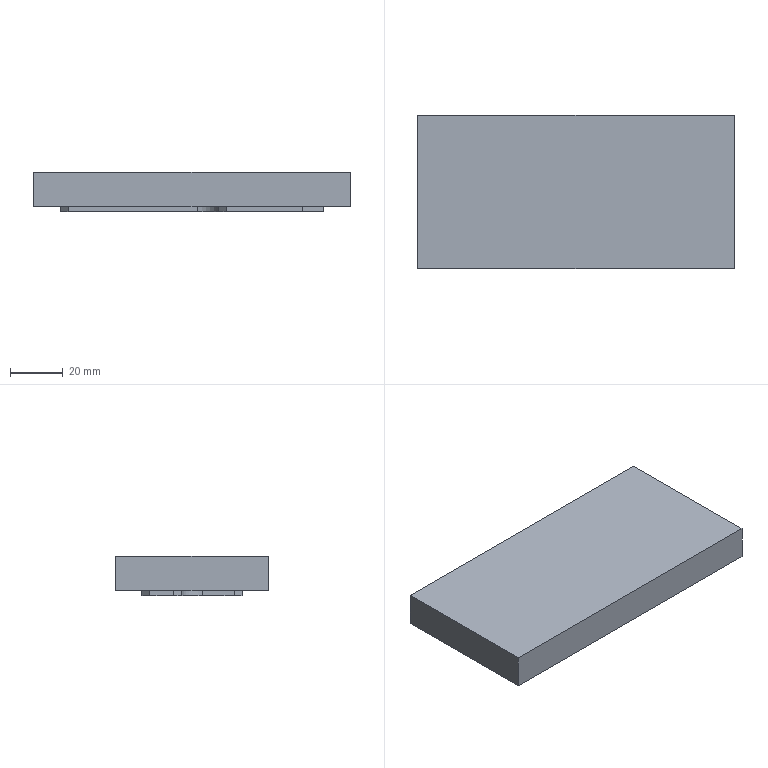NC program | NX | posted with a generic post | part box 120 x 58 x 15 mm
Lines 1 to 952 of 3687:
N10 G17 G21 G94 G90
(FLOOR_WALL_COPY , TOOL : D63)
N12 T03 M6
N14 G54
N16 G17 G0 G90 X-84.499 Y0. S6500 M3
N18 G43 Z30. H3
N20 Z3.
N22 G94 G1 Z0. F1250.
N24 X-81.499
N26 X81.499
N28 X84.499
N30 Z3.
N32 G0 Z30.
N34 M5
(DRILLING_COPY_1 , TOOL : D6A45)
N36 T01 M6
N38 G54
N40 G17 G0 G90 X30. Y0. S5000 M3
N42 G43 Z30. H1
N44 G94 G81 G98 Z-1. F250. R3.
N46 G80
N48 G0 X30. Y0. Z30.
N50 M5
(DRILLING_COPY_1_COPY , TOOL : 3.4ZT)
N52 T13 M6
N54 G54
N56 G17 G0 G90 X30. Y0. S2000 M3
N58 G43 Z30. H13
N60 G94 G83 G98 Z-7.521 F150. Q2. R3.
N62 G80
N64 G0 X30. Y0. Z30.
N66 M5
(ADAPTIVE_MILLING_COPY , TOOL : D10)
N68 T04 M6
N70 G54
N72 G17 G0 G90 X-60.77 Y7.063 S9500 M3
N74 G43 Z30. H4
N76 Z-4.
N78 G94 G1 Z-5. F1000.
N80 X-59.299 Y6.604 F3500.
N82 G3 X-58.124 Y7.063 R1.017
N84 X-57.341 Y9.86 R6.974
N86 X-57.022 Y18.975 R89.267
N88 G2 X-54.738 Y23.236 R5.593
N90 X-49.228 Y25.441 R11.859
N92 X-40.626 Y25.956 R58.355
N94 G1 X-39.751 Y25.965
N96 X-38.501 Y25.973
N98 X-36.876 Y25.98
N100 X-34.501 Y25.985
N102 X-30.501 Y25.987
N104 X-14.376 Y25.988
N106 X49.999
N108 X50.124 Y25.986
N110 X50.248 Y25.98
N112 X50.373 Y25.971
N114 G2 X54.621 Y23.182 R5.966
N116 X56.542 Y17.553 R13.282
N118 X56.959 Y9.319 R68.159
N120 G1 X56.968 Y8.194
N122 X56.976 Y6.694
N124 X56.982 Y4.694
N126 X56.986 Y1.694
N128 X56.988 Y-4.681
N130 Y-19.056
N132 G2 X54.74 Y-23.209 R5.607
N134 X49.361 Y-25.413 R11.758
N136 X41.012 Y-25.952 R54.734
N138 G1 X40.012 Y-25.963
N140 X38.762 Y-25.972
N142 X37.387 Y-25.978
N144 X35.262 Y-25.983
N146 X31.887 Y-25.987
N148 X23.262 Y-25.988
N150 X-49.988
N152 X-50.113 Y-25.987
N154 X-50.238 Y-25.981
N156 X-50.362 Y-25.974
N158 G2 X-54.616 Y-23.192 R5.973
N160 X-56.537 Y-17.564 R13.138
N162 X-56.964 Y-8.83 R72.275
N164 X-56.95 Y4.419 R472.203
N166 G3 X-56.269 Y11.259 R263.081
N168 G2 X-56.022 Y16.877 R317.639
N170 X-51.965 Y22.581 R7.959
N172 X-45.426 Y24.543 R16.784
N174 X-35.565 Y24.956 R91.928
N176 G1 X-34.065 Y24.964
N178 X-32.19 Y24.97
N180 X-29.44 Y24.974
N182 X-24.44 Y24.977
N184 X17.435 Y24.978
N186 X46.935
N188 G2 X53.285 Y21.359 R7.609
N190 X55.474 Y14.903 R15.425
N192 X55.952 Y4.921 R81.68
N194 G1 X55.96 Y3.671
N196 X55.967 Y2.046
N198 X55.972 Y-0.204
N200 X55.975 Y-3.954
N202 X55.977 Y-13.454
N204 Y-15.829
N206 G2 X52.343 Y-22.294 R7.594
N208 X46.007 Y-24.458 R15.35
N210 X36.901 Y-24.944 R73.284
N212 G1 X35.776 Y-24.954
N214 X34.401 Y-24.962
N216 X32.526 Y-24.969
N218 X29.901 Y-24.974
N220 X25.401 Y-24.977
N222 X5.651 Y-24.978
N224 X-46.849
N226 X-47.099 Y-24.975
N228 X-47.348 Y-24.966
N230 G2 X-53.375 Y-21.225 R7.67
N232 X-55.494 Y-14.742 R15.836
N234 X-55.947 Y-5.509 R78.791
N236 X-55.883 Y3.739 R153.277
N238 G3 X-55.15 Y14.19 R284.904
N240 G2 X-54.948 Y17.397 R13.758
N242 X-53.617 Y19.666 R6.048
N244 G1 X-50.666 Y22.617
N246 X-50.614 Y22.663
N248 G2 X-47.034 Y24.145 R5.569
N250 G1 X-46.965 Y24.15
N252 X41.965
N254 X42.284 Y24.131
N256 G2 X46.271 Y23.863 R31.993
N258 X52.517 Y19.095 R9.124
N260 X54.269 Y13.906 R17.717
N262 X55.15 Y10.965 R6.08
N264 G1 Y-10.965
N266 X55.131 Y-11.284
N268 G2 X54.865 Y-15.271 R32.332
N270 X50.095 Y-21.516 R9.13
N272 X44.906 Y-23.267 R17.748
N274 X41.965 Y-24.15 R6.061
N276 G1 X13.035
N278 X12.716 Y-24.131
N280 G3 X1.343 Y-23.991 R289.988
N282 G1 X-4.157 Y-23.989
N284 X-43.907 Y-23.988
N286 X-44.282 Y-23.987
N288 X-44.532 Y-23.983
N290 X-44.782 Y-23.976
N292 X-45.032 Y-23.964
N294 G2 X-52.461 Y-19.173 R8.944
N296 X-54.49 Y-12.262 R18.322
N298 X-54.94 Y-1.902 R97.025
N300 X-54.741 Y4.967 R90.693
N302 G3 X-54.984 Y5.736 R7.847
N304 G1 X-55.145 Y6.966
N306 X-55.15 Y7.035
N308 Y14.285
N310 G3 X-55.825 Y15.237 R1.031
N312 G1 X-57.636 Y16.086 Z-4.9
N314 G2 X-58.22 Y16.5 R1.32
N316 X-58.332 Y17.467 R1.014
N318 G1 X-57.686 Y18.999
N320 G2 X-56.569 Y20.732 R8.308
N322 G1 X-55.142 Y22.429
N324 X-53.699 Y24.114
N326 G2 X-46.012 Y27.459 R10.495
N328 G1 X38.853 Y27.327
N330 G2 X39.664 Y26.91 R1.015
N332 G1 X39.835 Y26.672
N334 X41. Y25.046 Z-5.
N336 X41.458 Y24.43
N338 G3 X42.034 Y24.145 R1.041
N340 G2 X43.978 Y23.717 R5.584
N342 X49.072 Y20.896 R13.089
N344 X52.204 Y16.124 R13.957
N346 G3 X53.663 Y14.614 R30.408
N348 G1 X54.418 Y13.63
N350 G3 X56.046 Y15.099 R-1.1
N352 G1 X44.92 Y25.62
N354 G3 X43.744 Y23.804 R-1.1
N356 G2 X45.614 Y22.663 R5.475
N358 X48.392 Y19.891 R26.386
N360 G1 X52.37 Y15.913
N362 G3 X53.926 Y15.916 R1.1
N364 X53.926 Y17.469 R1.1
N366 G1 X47.222 Y24.173
N368 G3 X45.666 Y24.17 R1.1
N370 X45.666 Y22.617 R1.1
N372 G1 X48.406 Y19.877
N374 G3 X49.312 Y19.604 R1.014
N376 G1 X49.758 Y19.695
N378 X51.718 Y20.093 Z-4.9
N380 X52.02 Y20.153
N382 X52.327 Y20.162
N384 G2 X52.906 Y19.877 R1.041
N386 G1 X54.411 Y18.379
N388 X55.9 Y16.865
N390 G2 X57.427 Y14.52 R8.704
N392 X57.853 Y12.935 R6.611
N394 X58.196 Y8.593 R32.631
N396 G1 X58.327 Y-7.853
N398 G2 X57.908 Y-8.675 R1.015
N400 G1 X57.663 Y-8.849
N402 X56.035 Y-10.01 Z-5.
N404 X55.431 Y-10.456
N406 G3 X55.145 Y-11.034 R1.041
N408 G2 X54.717 Y-12.978 R5.604
N410 X51.721 Y-18.252 R12.905
N412 X47.124 Y-21.203 R14.175
N414 G3 X45.614 Y-22.663 R38.251
N416 G1 X44.63 Y-23.418
N418 G3 X46.099 Y-25.046 R-1.1
N420 G1 X56.62 Y-13.92
N422 G3 X54.804 Y-12.744 R-1.1
N424 G2 X53.663 Y-14.614 R5.475
N426 X50.899 Y-17.385 R26.372
N428 G1 X46.921 Y-21.362
N430 G3 X46.924 Y-22.918 R1.1
N432 X48.477 Y-22.918 R1.1
N434 G1 X55.173 Y-16.222
N436 G3 X55.17 Y-14.666 R1.1
N438 X53.617 Y-14.666 R1.1
N440 G1 X50.877 Y-17.406
N442 G3 X50.604 Y-18.312 R1.014
N444 G1 X50.695 Y-18.758
N446 X51.093 Y-20.718 Z-4.9
N448 X51.153 Y-21.02
N450 X51.162 Y-21.327
N452 G2 X50.877 Y-21.906 R1.041
N454 G1 X49.378 Y-23.411
N456 X47.865 Y-24.9
N458 G2 X45.527 Y-26.438 R8.747
N460 X43.943 Y-26.86 R6.375
N462 X39.604 Y-27.184 R33.85
N464 G1 X16.147 Y-27.327
N466 G2 X15.327 Y-26.908 R1.015
N468 G1 X15.153 Y-26.664
N470 X13.991 Y-25.035 Z-5.
N472 X13.543 Y-24.431
N474 G3 X12.966 Y-24.145 R1.041
N476 G2 X10.776 Y-23.664 R7.313
N478 G3 X5.066 Y-23.086 R28.083
N480 X-8.058 Y-23. R693.381
N482 G1 X-22.933 Y-22.999
N484 X-40.933
N486 X-41.683 Y-22.995
N488 X-42.183 Y-22.989
N490 X-42.433 Y-22.984
N492 G2 X-51.504 Y-17.387 R9.93
N494 X-53.507 Y-9.948 R20.904
N496 X-53.824 Y3.164 R106.776
N498 G3 X-54.003 Y3.829 R1.592
N500 G2 X-54.822 Y5.298 R4.129
N502 G3 X-56.425 Y5.648 R1.002
N504 X-56.759 Y4.813 Z-4.954 R1.158
N506 G1 X-56.858 Y3.743 Z-4.9
N508 X-57.072 Y1.401
N510 X-57.076 Y-2.482
N512 X-57.059 Y-6.364
N514 G3 X-56.336 Y-12.277 R32.958
N516 X-54.971 Y-17.07 R31.668
N518 G1 X-54.579 Y-18.122
N520 X-54.141 Y-19.155
N522 G3 X-51.732 Y-22.28 R9.329
N524 G1 X-50.149 Y-23.575
N526 G3 X-43.587 Y-26.137 R13.27
N528 G1 X-42.948 Y-26.188
N530 X-42.307 Y-26.217
N532 X8.19 Y-27.034
N534 X8.408 Y-27.01
N536 X8.618 Y-26.946
N538 X10.364 Y-26.156
N540 X10.963 Y-25.891 Z-4.933
N542 X11.551 Y-25.603 Z-4.966
N544 G3 X11.949 Y-25.056 Z-5. R1.038
N546 X11.372 Y-23.852 R1.005
N548 G1 X9.345 Y-22.959
N550 G3 X3.666 Y-22.165 R22.692
N552 X-14.957 Y-22.01 R532.866
N554 G1 X-37.832
N556 X-38.957 Y-22.003
N558 X-39.957 Y-21.995
N560 X-40.332 Y-21.99
N562 X-40.582 Y-21.984
N564 G2 X-47.346 Y-19.78 R10.87
N566 X-51.473 Y-13.358 R12.917
N568 X-52.747 Y-4.725 R34.9
N570 X-52.857 Y1.648 R370.505
N572 G3 X-53.663 Y3.386 R2.026
N574 G1 X-54.043 Y3.882
N576 G3 X-55.346 Y4.133 R1.005
N578 X-55.852 Y3.229 Z-4.946 R1.107
N580 G1 X-55.979 Y2.319 Z-4.9
N582 X-56.144 Y1.153
N584 X-56.293 Y-0.015
N586 X-56.295 Y-1.701
N588 X-56.248 Y-3.386
N590 X-56.15 Y-4.505
N592 X-56.008 Y-5.618
N594 X-55.564 Y-8.529
N596 X-55.099 Y-11.437
N598 G3 X-53.19 Y-17.642 R29.483
N600 X-50.157 Y-21.539 R10.754
N602 X-44.6 Y-24.547 R16.231
N604 X-41.067 Y-25.08 R13.269
N606 G1 X6.473 Y-25.668
N608 X6.623 Y-25.658
N610 X8.786 Y-25.357
N612 X10.042 Y-25.171 Z-4.964
N614 G3 X10.61 Y-24.739 Z-5. R1.031
N616 X10.37 Y-23.418 R1.005
N618 X6.54 Y-21.707 R7.6
N620 X-1.177 Y-21.096 R47.61
N622 X-15.176 Y-21.022 R740.994
N624 G1 X-28.051 Y-21.021
N626 X-34.926
N628 X-36.051 Y-21.014
N630 X-38.051 Y-20.998
N632 G2 X-43.802 Y-20.023 R14.432
N634 X-49.601 Y-14.076 R11.504
N636 X-51.496 Y-6.213 R24.432
N638 X-51.837 Y0.276 R157.843
N640 G3 X-52.168 Y1.854 R3.925
N642 G1 X-52.247 Y1.964
N644 X-53.219 Y2.936
N646 G3 X-54.412 Y3.103 R1.007
N648 X-54.944 Y2.223 Z-4.947 R1.111
N650 G1 X-55.108 Y1.309 Z-4.9
N652 X-55.304 Y0.251
N654 X-55.477 Y-0.811
N656 X-55.469 Y-0.961
N658 X-54.47 Y-9.024
N660 G3 X-53.31 Y-13.338 R16.538
N662 X-52.026 Y-16.042 R27.7
N664 G1 X-51.472 Y-17.057
N666 X-50.876 Y-18.048
N668 G3 X-46.132 Y-22.198 R12.311
N670 X-42.785 Y-23.537 R16.846
N672 X-40.82 Y-23.81 R9.452
N674 G1 X5.778 Y-25.135
N676 X5.946 Y-25.126
N678 X8.075 Y-24.827
N680 X8.726 Y-24.741 Z-4.933
N682 X9.373 Y-24.63 Z-4.966
N684 G3 X9.907 Y-24.22 Z-5. R1.039
N686 X9.676 Y-22.885 R1.005
N688 X8.471 Y-21.901 R18.398
N690 X4.195 Y-20.593 R11.784
N692 X-5.659 Y-20.072 R78.464
N694 G1 X-6.784 Y-20.061
N696 X-8.159 Y-20.052
N698 X-9.909 Y-20.044
N700 X-12.284 Y-20.038
N702 X-15.784 Y-20.034
N704 X-22.784 Y-20.032
N706 G2 X-38.033 Y-19.944 R507.107
N708 X-48.344 Y-13.18 R11.597
N710 X-50.443 Y-4.863 R23.851
N712 G3 X-50.941 Y0.235 R59.396
N714 X-51.23 Y0.947 R1.91
N716 G1 X-52.29 Y2.007
N718 G3 X-53.477 Y2.178 R1.007
N720 X-54.015 Y1.302 Z-4.947 R1.111
N722 G1 X-54.185 Y0.389 Z-4.9
N724 X-54.557 Y-1.64
N726 X-54.54 Y-1.89
N728 X-54.064 Y-4.341
N730 X-53.539 Y-6.781
N732 G3 X-51.894 Y-12.805 R135.046
N734 X-49.422 Y-17.385 R14.016
N736 G1 X-48.89 Y-17.98
N738 X-48.327 Y-18.544
N740 X-47.481 Y-19.332
N742 X-46.6 Y-20.082
N744 G3 X-43.183 Y-21.906 R12.408
N746 X-39.312 Y-22.788 R18.17
N748 G1 X-38.197 Y-22.901
N750 X-37.079 Y-22.973
N752 X5.276 Y-24.6
N754 X7.397 Y-24.24
N756 X8.049 Y-24.133 Z-4.933
N758 X8.696 Y-24.002 Z-4.966
N760 G3 X9.213 Y-23.583 Z-5. R1.039
N762 X9.069 Y-22.352 R1.007
N764 X5.257 Y-20.109 R6.986
N766 X-1.924 Y-19.219 R34.451
N768 X-20.922 Y-19.043 R549.983
N770 G2 X-36.296 Y-18.952 R636.005
N772 X-43.243 Y-16.805 R12.733
N774 X-48.09 Y-9.992 R13.604
N776 X-49.47 Y-3.144 R32.232
N778 G3 X-50.046 Y-0.21 R11.948
N780 X-50.666 Y0.383 R2.633
N782 G1 X-51.285 Y1.002
N784 G3 X-52.461 Y1.178 R1.007
N786 X-53.009 Y0.31 Z-4.947 R1.112
N788 G1 X-53.193 Y-0.602 Z-4.9
N790 X-53.557 Y-2.411
N792 X-53.572 Y-2.655
N794 X-53.535 Y-2.895
N796 X-52.364 Y-6.83
N798 X-51.17 Y-10.758
N800 G3 X-48.512 Y-16.063 R21.966
N802 X-46.242 Y-18.41 R11.769
N804 X-42.701 Y-20.608 R16.968
N806 X-39.441 Y-21.55 R13.495
N808 X-36.469 Y-21.875 R25.511
N810 G1 X4.485 Y-23.806
N812 X6.601 Y-23.445
N814 X7.253 Y-23.338 Z-4.933
N816 X7.9 Y-23.206 Z-4.966
N818 G3 X8.418 Y-22.788 Z-5. R1.039
N820 X8.273 Y-21.556 R1.007
N822 X4.373 Y-19.216 R7.301
N824 X-3.174 Y-18.245 R35.148
N826 X-19.797 Y-18.056 R454.491
N828 G2 X-34.921 Y-17.944 R508.533
N830 X-41.997 Y-15.784 R13.258
N832 X-46.976 Y-8.916 R13.779
N834 X-48.405 Y-2.967 R40.966
N836 G3 X-49.073 Y-0.83 R6.777
N838 X-49.63 Y-0.418 R2.122
N840 G1 X-50.324 Y0.115
N842 G3 X-51.646 Y0.023 R1.005
N844 X-51.913 Y-0.902 Z-4.95 R1.037
N846 G1 X-51.789 Y-1.892 Z-4.9
N848 X-51.489 Y-4.232
N850 X-50.537 Y-7.986
N852 G3 X-47.34 Y-14.56 R20.824
N854 X-45.497 Y-16.919 R25.902
N856 X-41.825 Y-19.415 R10.104
N858 X-36.73 Y-20.743 R18.342
N860 G1 X-35.334 Y-20.892
N862 X-33.935 Y-20.997
N864 X3.693 Y-23.011
N866 X5.808 Y-22.65
N868 X6.459 Y-22.542 Z-4.933
N870 X7.106 Y-22.41 Z-4.966
N872 G3 X7.623 Y-21.991 Z-5. R1.039
N874 X7.478 Y-20.761 R1.007
N876 X3.257 Y-18.245 R7.744
N878 X-4.541 Y-17.262 R36.911
N880 X-23.164 Y-17.065 R511.304
N882 G2 X-33.912 Y-16.92 R269.318
N884 X-41.551 Y-14.188 R13.125
N886 X-46.004 Y-7.519 R14.606
N888 X-47.504 Y-2.489 R252.114
N890 G3 X-48.362 Y-0.99 R3.212
N892 G1 X-48.467 Y-0.922
N894 X-48.487 Y-0.911
N896 X-49.511 Y-0.487
N898 G3 X-50.57 Y-0.674 R1.011
N900 X-50.889 Y-1.547 Z-4.952 R1.044
N902 G1 X-50.845 Y-2.582 Z-4.9
N904 X-50.752 Y-4.586
N906 X-50.675 Y-4.833
N908 X-48.061 Y-10.511
N910 G3 X-44.946 Y-15.122 R17.871
N912 X-40.473 Y-18.406 R13.609
N914 X-35.086 Y-19.794 R14.929
N916 G1 X2.814 Y-22.127
N918 X4.923 Y-21.767
N920 X5.575 Y-21.659 Z-4.933
N922 X6.222 Y-21.526 Z-4.966
N924 G3 X6.739 Y-21.107 Z-5. R1.039
N926 X6.594 Y-19.877 R1.007
N928 X5.476 Y-18.716 R10.7
N930 X1.328 Y-17.058 R10.801
N932 X-7.12 Y-16.228 R49.786
N934 X-25.869 Y-16.048 R901.569
N936 G2 X-33.239 Y-15.86 R102.234
N938 X-44.016 Y-8.598 R12.836
N940 X-46.036 Y-3.621 R48.439
N942 G3 X-47.381 Y-1.249 R6.45
N944 X-48.397 Y-0.948 R2.47
N946 G1 X-48.513 Y-0.9
N948 G3 X-49.592 Y-1.107 R1.01
N950 X-49.893 Y-1.948 Z-4.954 R1.048
N952 G1 X-49.865 Y-3.024 Z-4.9
N954 X-49.82 Y-4.758
N956 X-49.777 Y-5.011
N958 X-49.677 Y-5.247
N960 X-45.176 Y-12.75
N962 G3 X-43.113 Y-15.044 R8.516
N964 X-38.82 Y-17.546 R19.198
N966 X-34.002 Y-18.698 R16.626
N968 X-26.528 Y-19.206 R183.169
N970 G1 X1.844 Y-20.488
N972 X4.061 Y-20.773
N974 X4.709 Y-20.861 Z-4.933
N976 X5.361 Y-20.924 Z-4.966
N978 G3 X5.987 Y-20.667 Z-5. R1.038
N980 X6.109 Y-19.316 R1.005
N982 X2.687 Y-16.749 R6.299
N984 X-4.175 Y-15.47 R26.746
N986 X-18.292 Y-15.096 R209.674
N988 G2 X-30.79 Y-14.944 R423.993
N990 X-37.849 Y-13.08 R15.223
N992 X-43.211 Y-7.121 R14.405
N994 G3 X-45.438 Y-2.646 R128.412
N996 X-46.653 Y-1.246 R3.646
N998 X-47.902 Y-1.031 R6.242
N1000 X-48.903 Y-1.53 R1.01
N1002 X-48.952 Y-2.427 Z-4.954 R1.048
N1004 G1 X-48.619 Y-3.444 Z-4.9
N1006 X-47.961 Y-5.424
N1008 X-46.138 Y-8.336
N1010 X-44.293 Y-11.233
N1012 G3 X-41.128 Y-14.731 R18.235
N1014 X-38.216 Y-16.386 R11.621
N1016 X-34.639 Y-17.444 R19.581
N1018 G1 X-33.406 Y-17.618
N1020 X-32.167 Y-17.742
N1022 G3 X-25.945 Y-18.234 R162.263
N1024 G1 X1.276 Y-19.798
N1026 X3.489 Y-20.015
N1028 X4.139 Y-20.084 Z-4.933
N1030 X4.792 Y-20.127 Z-4.965
N1032 G3 X5.41 Y-19.85 Z-5. R1.038
N1034 X5.582 Y-18.63 R1.007
N1036 X3.412 Y-16.459 R4.36
N1038 X-2.201 Y-14.825 R17.502
N1040 X-12.674 Y-14.178 R84.393
N1042 G2 X-29.297 Y-13.957 R993.749
N1044 X-36.177 Y-12.342 R16.272
N1046 X-41.9 Y-6.717 R14.953
N1048 G3 X-44.509 Y-2.455 R74.541
N1050 X-45.872 Y-1.202 R3.484
N1052 X-47.034 Y-1.145 R5.721
N1054 X-47.964 Y-1.64 R1.011
N1056 X-48.03 Y-2.524 Z-4.954 R1.049
N1058 G1 X-47.72 Y-3.563 Z-4.9
N1060 X-47.153 Y-5.442
N1062 X-47.034 Y-5.645
N1064 X-44.615 Y-8.848
N1066 G3 X-40.912 Y-12.679 R28.919
N1068 G1 X-40.035 Y-13.432
N1070 X-39.125 Y-14.145
N1072 G3 X-36.099 Y-15.677 R12.302
N1074 X-32.298 Y-16.619 R21.017
N1076 G1 X-30.909 Y-16.812
N1078 X-29.513 Y-16.957
N1080 X1.088 Y-19.446
N1082 X3.253 Y-19.585
N1084 X3.923 Y-19.633 Z-4.934
N1086 X4.594 Y-19.657 Z-4.967
N1088 G3 X5.18 Y-19.389 Z-5. R1.041
N1090 X5.418 Y-18.28 R1.01
N1092 X3.157 Y-15.724 R4.503
N1094 X-2.66 Y-13.913 R17.215
N1096 X-13.253 Y-13.202 R81.361
N1098 G2 X-28.126 Y-12.957 R855.934
N1100 X-35.008 Y-11.34 R16.746
N1102 X-40.618 Y-6.284 R16.031
N1104 G3 X-43.566 Y-2.249 R60.005
N1106 X-44.923 Y-1.179 R3.273
N1108 G1 X-46.21 Y-1.15
N1110 G3 X-47.175 Y-1.886 R1.007
N1112 X-46.916 Y-2.882 Z-4.946 R1.11
N1114 G1 X-46.377 Y-3.636 Z-4.9
N1116 X-45.046 Y-5.497
N1118 X-43.365 Y-7.748
N1120 X-41.664 Y-9.982
N1122 G3 X-38.42 Y-12.813 R13.405
N1124 X-33.346 Y-15.128 R18.305
N1126 X-30.909 Y-15.598 R17.204
N1128 G1 X-24.391 Y-16.337
N1130 X-17.866 Y-17.02
N1132 X0.866 Y-18.87
N1134 X3.001 Y-19.007
N1136 X3.676 Y-19.054 Z-4.934
N1138 X4.352 Y-19.08 Z-4.968
N1140 G3 X4.932 Y-18.82 Z-5. R1.042
N1142 X5.178 Y-17.702 R1.01
N1144 X3.07 Y-15.063 R4.421
N1146 X-2.56 Y-13.093 R16.044
N1148 X-12.765 Y-12.251 R68.656
N1150 G1 X-13.765 Y-12.225
N1152 X-14.765 Y-12.204
N1154 X-15.765 Y-12.185
N1156 X-16.765 Y-12.168
N1158 X-20.014 Y-12.121
N1160 X-22.889 Y-12.082
N1162 X-24.014 Y-12.06
N1164 X-25.263 Y-12.031
N1166 G2 X-31.81 Y-11.17 R24.127
N1168 X-38.94 Y-6.298 R15.678
N1170 G3 X-42.413 Y-2.198 R131.781
N1172 X-43.808 Y-1.174 R3.497
N1174 G1 X-43.947 Y-1.15
N1176 X-45.197
N1178 G3 X-46.162 Y-1.886 R1.007
N1180 X-45.903 Y-2.883 Z-4.946 R1.11
N1182 G1 X-45.364 Y-3.636 Z-4.9
N1184 X-44.397 Y-4.99
N1186 X-43.444 Y-6.353
N1188 X-43.174 Y-6.669
N1190 X-42.889 Y-6.97
N1192 X-41.271 Y-8.532
N1194 X-39.639 Y-10.079
N1196 G3 X-33.359 Y-13.791 R18.313
N1198 X-29.723 Y-14.604 R18.841
N1200 X-24.763 Y-15.17 R85.364
N1202 G1 X0.516 Y-17.264
N1204 X0.763 Y-17.316
N1206 X2.602 Y-17.957
N1208 X3.226 Y-18.18 Z-4.933
N1210 X3.859 Y-18.38 Z-4.966
N1212 G3 X4.509 Y-18.269 Z-5. R1.04
N1214 X5.016 Y-17.264 R1.01
N1216 X3.702 Y-14.935 R3.367
N1218 X-1.095 Y-12.612 R12.039
N1220 X-9.998 Y-11.411 R43.369
N1222 X-24.992 Y-11.01 R862.651
N1224 G2 X-32.19 Y-9.616 R20.049
N1226 X-38.207 Y-5.227 R18.406
N1228 G3 X-41.718 Y-1.672 R45.853
N1230 X-42.709 Y-1.15 R2.051
N1232 G1 X-43.959
N1234 G3 X-44.922 Y-1.881 R1.007
N1236 X-44.669 Y-2.878 Z-4.947 R1.111
N1238 G1 X-44.134 Y-3.637 Z-4.9
N1240 X-42.869 Y-5.42
N1242 G3 X-39.285 Y-8.587 R64.471
N1244 G1 X-38.125 Y-9.488
N1246 X-36.952 Y-10.372
N1248 G3 X-30.171 Y-13.362 R18.149
N1250 X-27.22 Y-13.848 R29.329
N1252 G1 X0.578 Y-16.911
N1254 X2.533 Y-17.581
N1256 X3.167 Y-17.806 Z-4.934
N1258 X3.807 Y-18.008 Z-4.967
N1260 G3 X4.443 Y-17.907 Z-5. R1.041
N1262 X4.967 Y-16.892 R1.01
N1264 X3.472 Y-14.117 R3.811
N1266 X-1.67 Y-11.653 R12.921
N1268 X-11.072 Y-10.416 R46.3
N1270 X-23.441 Y-10.045 R816.021
N1272 G2 X-30.56 Y-8.844 R23.011
N1274 X-37.302 Y-4.412 R20.151
N1276 G3 X-40.673 Y-1.436 R34.841
N1278 X-41.358 Y-1.15 R1.793
N1280 G1 X-42.733
N1282 G3 X-43.695 Y-1.876 R1.007
N1284 X-43.449 Y-2.872 Z-4.947 R1.112
N1286 G1 X-42.92 Y-3.637 Z-4.9
N1288 X-41.791 Y-5.266
N1290 X-41.686 Y-5.387
N1292 X-41.569 Y-5.497
N1294 X-39.671 Y-6.922
N1296 X-37.761 Y-8.333
N1298 G3 X-32.695 Y-11.265 R32.991
N1300 X-28.892 Y-12.438 R19.125
N1302 G1 X-27.788 Y-12.644
N1304 X-26.678 Y-12.813
N1306 X0.487 Y-16.291
N1308 X2.443 Y-16.96
N1310 X3.081 Y-17.185 Z-4.934
N1312 X3.725 Y-17.388 Z-4.968
N1314 G3 X4.354 Y-17.291 Z-5. R1.042
N1316 X4.886 Y-16.272 R1.007
N1318 X3.51 Y-13.507 R3.757
N1320 X-1.428 Y-10.915 R12.406
N1322 X-10.675 Y-9.503 R41.637
N1324 X-22.791 Y-9.044 R778.734
N1326 G2 X-30.58 Y-7.43 R21.973
N1328 X-36.71 Y-3.379 R24.878
N1330 G3 X-39.489 Y-1.26 R21.935
N1332 G1 X-39.604 Y-1.212
N1334 X-39.724 Y-1.177
N1336 X-39.847 Y-1.154
N1338 X-39.879 Y-1.15
N1340 X-41.379
N1342 G3 X-42.337 Y-1.865 R1.007
N1344 X-42.105 Y-2.862 Z-4.947 R1.113
N1346 G1 X-41.585 Y-3.637 Z-4.9
N1348 X-41.027 Y-4.479
N1350 X-40.45 Y-5.307
N1352 X-40.214 Y-5.497
N1354 X-36.92 Y-7.409
N1356 X-33.613 Y-9.299
N1358 G3 X-27.282 Y-11.459 R20.546
N1360 G1 X-17.956 Y-12.973
N1362 X-11.857 Y-13.949
N1364 X0.35 Y-15.84
N1366 X1.361 Y-16.131
N1368 X2.368 Y-16.438
N1370 X3.036 Y-16.643 Z-4.935
N1372 X3.709 Y-16.83 Z-4.97
N1374 G3 X4.295 Y-16.736 Z-5. R1.048
N1376 X4.85 Y-15.84 R1.011
N1378 X3.708 Y-13.038 R3.576
N1380 X-1.095 Y-10.217 R11.753
N1382 X-10.055 Y-8.616 R37.346
N1384 X-21.791 Y-8.064 R505.358
N1386 G2 X-30.047 Y-6.26 R23.131
N1388 X-36.164 Y-2.399 R32.046
N1390 G3 X-38.056 Y-1.193 R10.528
N1392 X-39.903 Y-1.15 R12.21
N1394 X-40.898 Y-2.243 R1.004
N1396 X-40.418 Y-3.013 Z-4.953 R1.046
N1398 G1 X-39.563 Y-3.641 Z-4.9
N1400 X-37.095 Y-5.45
N1402 X-34.607 Y-7.234
N1404 G3 X-30.502 Y-9.296 R19.757
N1406 X-24.727 Y-10.838 R33.857
N1408 G1 X0.461 Y-15.367
N1410 X2.334 Y-15.929
N1412 X3.702 Y-16.329 Z-4.971
N1414 G3 X4.263 Y-16.251 Z-5. R1.053
N1416 X4.85 Y-15.34 R1.01
N1418 X3.665 Y-12.295 R3.84
N1420 X-1.218 Y-9.366 R12.037
N1422 X-10.286 Y-7.669 R37.516
N1424 X-21.269 Y-7.054 R895.504
N1426 G2 X-33.637 Y-2.8 R23.815
N1428 G3 X-36.306 Y-1.186 R18.036
N1430 X-38.372 Y-1.15 R18.719
N1432 X-39.305 Y-2.834 R1.102
N1434 X-38.507 Y-3.357 Z-4.951 R1.237
N1436 G1 X-37.53 Y-3.646 Z-4.9
N1438 X2.334 Y-15.443
N1440 X2.966 Y-15.634 Z-4.933
N1442 X3.604 Y-15.805 Z-4.966
N1444 G3 X4.261 Y-15.689 Z-5. R1.146
N1446 X4.85 Y-14.715 R1.112
N1448 X3.642 Y-11.549 R3.99
N1450 X-1.44 Y-8.469 R12.566
N1452 X-10.375 Y-6.734 R37.461
N1454 X-20.477 Y-6.072 R905.08
N1456 G2 X-32.268 Y-2.297 R25.921
N1458 G3 X-34.359 Y-1.18 R17.8
N1460 X-36.524 Y-1.15 R43.042
N1462 X-37.445 Y-2.851 R1.102
N1464 X-36.651 Y-3.359 Z-4.952 R1.244
N1466 G1 X-35.66 Y-3.647 Z-4.9
N1468 X2.333 Y-14.699
N1470 X2.968 Y-14.887 Z-4.933
N1472 X3.608 Y-15.056 Z-4.966
N1474 G3 X4.262 Y-14.939 Z-5. R1.147
N1476 X4.85 Y-13.965 R1.112
N1478 X3.629 Y-10.799 R4.077
N1480 X-1.414 Y-7.653 R12.717
N1482 X-10.452 Y-5.803 R36.765
N1484 G1 X-10.95 Y-5.755
N1486 X-11.448 Y-5.71
N1488 X-11.946 Y-5.668
N1490 X-12.569 Y-5.619
N1492 X-13.317 Y-5.564
N1494 X-14.19 Y-5.504
N1496 X-15.936 Y-5.39
N1498 X-17.308 Y-5.292
N1500 X-18.056 Y-5.238
N1502 X-18.803 Y-5.178
N1504 X-19.301 Y-5.134
N1506 X-19.799 Y-5.086
N1508 X-19.923 Y-5.073
N1510 G2 X-31.307 Y-1.551 R29.578
N1512 G3 X-32.311 Y-1.15 R4.037
N1514 G1 X-34.561
N1516 G3 X-35.478 Y-2.858 R1.102
N1518 X-34.685 Y-3.359 Z-4.952 R1.247
N1520 G1 X-33.689 Y-3.647 Z-4.9
N1522 X2.333 Y-14.075
N1524 X2.968 Y-14.263 Z-4.933
N1526 X3.609 Y-14.431 Z-4.966
N1528 G3 X4.262 Y-14.314 Z-5. R1.147
N1530 X4.85 Y-13.34 R1.112
N1532 X3.627 Y-10.046 R4.2
N1534 X-1.494 Y-6.792 R12.905
N1536 X-10.641 Y-4.858 R37.041
N1538 G2 X-19.976 Y-3.998 R362.915
N1540 X-29.535 Y-1.196 R33.777
N1542 G1 X-29.656 Y-1.166
N1544 X-29.771 Y-1.15
N1546 X-32.396
N1548 G3 X-33.304 Y-2.871 R1.101
N1550 X-32.515 Y-3.36 Z-4.952 R1.253
N1552 G1 X-31.508 Y-3.648 Z-4.9
N1554 X2.332 Y-13.329
N1556 X2.969 Y-13.515 Z-4.933
N1558 X3.612 Y-13.682 Z-4.966
N1560 G3 X4.263 Y-13.563 Z-5. R1.147
N1562 X4.85 Y-12.59 R1.112
N1564 X3.633 Y-9.29 R4.272
N1566 X-1.565 Y-5.929 R13.04
N1568 X-10.945 Y-3.897 R37.441
N1570 G2 X-20.015 Y-2.91 R184.531
N1572 X-26.654 Y-1.164 R37.11
N1574 G1 X-26.752 Y-1.15
N1576 X-29.877
N1578 G3 X-30.782 Y-2.876 R1.101
N1580 X-29.995 Y-3.36 Z-4.953 R1.256
N1582 G1 X-28.983 Y-3.649 Z-4.9
N1584 X2.332 Y-12.58
N1586 X2.97 Y-12.765 Z-4.933
N1588 X3.613 Y-12.932 Z-4.966
N1590 G3 X4.263 Y-12.813 Z-5. R1.147
N1592 X4.85 Y-11.84 R1.112
N1594 X3.651 Y-8.531 R4.321
N1596 X-1.278 Y-5.206 R12.909
N1598 X-10.494 Y-3.019 R35.688
N1600 G2 X-19.425 Y-1.919 R190.75
N1602 X-22.975 Y-1.15 R83.288
N1604 G1 X-26.85
N1606 G3 X-27.762 Y-2.866 R1.101
N1608 X-26.973 Y-3.36 Z-4.952 R1.252
N1610 G1 X-25.969 Y-3.65 Z-4.9
N1612 X2.332 Y-11.826
N1614 X2.968 Y-12.013 Z-4.933
N1616 X3.609 Y-12.181 Z-4.966
N1618 G3 X4.262 Y-12.064 Z-5. R1.147
N1620 X4.85 Y-11.09 R1.112
N1622 X3.593 Y-7.675 R4.43
N1624 X-1.447 Y-4.292 R13.344
N1626 X-10.655 Y-2.066 R36.709
N1628 G1 X-11.151 Y-2.
N1630 X-12.019 Y-1.89
N1632 X-13.26 Y-1.738
N1634 X-13.632 Y-1.692
N1636 X-14.624 Y-1.566
N1638 X-15.615 Y-1.436
N1640 X-16.235 Y-1.353
N1642 X-16.854 Y-1.266
N1644 X-17.348 Y-1.19
N1646 X-17.597 Y-1.15
N1648 X-23.097
N1650 G3 X-24.032 Y-2.828 R1.102
N1652 X-23.237 Y-3.357 Z-4.951 R1.236
N1654 G1 X-22.262 Y-3.65 Z-4.9
N1656 X2.332 Y-11.062
N1658 X2.962 Y-11.256 Z-4.933
N1660 X3.599 Y-11.43 Z-4.966
N1662 G3 X4.258 Y-11.316 Z-5. R1.146
N1664 X4.85 Y-10.34 R1.112
N1666 X3.624 Y-6.911 R4.482
N1668 X-1.609 Y-3.373 R13.634
N1670 X-10.529 Y-1.15 R37.551
N1672 G1 X-17.654
N1674 G3 X-18.653 Y-2.712 R1.102
N1676 X-17.836 Y-3.351 Z-4.946 R1.217
N1678 G1 X-16.959 Y-3.651 Z-4.9
N1680 X2.333 Y-10.267
N1682 X2.944 Y-10.482 Z-4.932
N1684 X3.563 Y-10.674 Z-4.965
N1686 G3 X4.247 Y-10.572 Z-5. R1.144
N1688 X4.85 Y-9.59 R1.112
N1690 X3.659 Y-6.147 R4.506
N1692 X-1.533 Y-2.549 R13.616
N1694 X-5.818 Y-1.15 R29.016
N1696 G1 X-10.568
N1698 G3 X-11.644 Y-2.481 R1.103
N1700 X-10.932 Y-3.292 Z-4.944 R1.133
N1702 G1 X-10.136 Y-3.652 Z-4.9
N1704 X2.335 Y-9.283
N1706 X3.445 Y-9.772 Z-4.961
N1708 G3 X4.213 Y-9.713 Z-5. R1.132
N1710 X4.85 Y-8.715 R1.111
N1712 X3.621 Y-5.284 R4.551
N1714 X-1.567 Y-1.677 R13.826
N1716 X-2.987 Y-1.15 R9.637
N1718 G1 X-5.862
N1720 G3 X-6.961 Y-2.282 R1.104
N1722 X-6.338 Y-3.246 Z-4.94 R1.128
N1724 G1 X-5.655 Y-3.653 Z-4.9
N1726 X2.337 Y-8.405
N1728 X2.833 Y-8.703 Z-4.929
N1730 X3.339 Y-8.985 Z-4.958
N1732 G3 X4.16 Y-8.986 Z-5. R1.129
N1734 X4.85 Y-7.965 R1.108
N1736 X3.586 Y-4.419 R4.649
N1738 X-0.811 Y-1.19 R12.78
N1740 X-3.023 Y-1.15 R16.427
N1742 X-4.118 Y-2.149 R1.106
N1744 X-3.596 Y-3.194 Z-4.939 R1.125
N1746 G1 X-2.974 Y-3.65 Z-4.9
N1748 X2.335 Y-7.542
N1750 X2.786 Y-7.876 Z-4.928
N1752 X3.249 Y-8.194 Z-4.956
N1754 G3 X4.1 Y-8.258 Z-5. R1.128
N1756 X4.85 Y-7.215 R1.108
N1758 X3.557 Y-3.553 R4.748
N1760 X0.675 Y-1.197 R9.098
N1762 X-1.066 Y-1.15 R10.19
N1764 X-1.778 Y-3.088 R1.101
N1766 G1 X3.038 Y-7.179
N1768 G3 X4.85 Y-6.34 R1.101
N1770 X3.612 Y-2.782 R4.705
N1772 X1.853 Y-1.215 R5.653
N1774 X0.32 Y-1.15 R6.033
N1776 X-0.432 Y-3.052 R1.101
N1778 G1 X2.998 Y-6.268
N1780 G3 X4.85 Y-5.465 R1.101
N1782 X2.925 Y-1.347 R4.672
N1784 X1.541 Y-1.15 R3.927
N1786 X0.722 Y-2.984 R1.101
N1788 G1 X2.931 Y-5.449
N1790 G3 X4.85 Y-4.715 R1.101
N1792 X4.187 Y-2.206 R3.535
N1794 X2.591 Y-1.244 R2.817
N1796 X1.672 Y-3.137 R1.101
N1798 G1 X2.905 Y-4.279
N1800 G3 X4.708 Y-3.164 R1.1
N1802 X2.776 Y-3.682 R1.151
N1804 G1 Z-2.
N1806 G0 Z30.
N1808 M5
(ZLEVEL_PROFILE_1_COPY , TOOL : D6JING)
N1810 T16 M6
N1812 G54
N1814 G17 G0 G90 X-47.658 Y22.539 S9500 M3
N1816 G43 Z30. H16
N1818 Z-4.
N1820 G94 G1 Z-5. F1000.
N1822 X-47.52 Y22.3
N1824 G3 X-47. Y22. R0.6
N1826 G1 X42.
N1828 G2 X44.121 Y21.121 R3.
N1830 G1 X52.121 Y13.121
N1832 G2 X53. Y11. R3.
N1834 G1 Y-11.
N1836 G2 X52.121 Y-13.121 R3.
N1838 G1 X44.121 Y-21.121
N1840 G2 X42. Y-22. R3.
N1842 G1 X13.
N1844 G2 X10.879 Y-21.121 R3.
N1846 G1 X7.879 Y-18.121
N1848 G2 X7. Y-16. R3.
N1850 G1 Y-4.
N1852 G3 X2. Y1. R5.
N1854 G1 X-47.
N1856 G2 X-49.121 Y1.879 R3.
N1858 G1 X-52.121 Y4.879
N1860 G2 X-53. Y7. R3.
N1862 G1 Y16.
N1864 G2 X-52.121 Y18.121 R3.
N1866 G1 X-49.121 Y21.121
N1868 G2 X-47. Y22. R3.
N1870 G3 X-46.48 Y22.3 R0.6
N1872 G1 X-46.307 Y22.6
N1874 Z-4.
N1876 G0 Z30.
N1878 M5